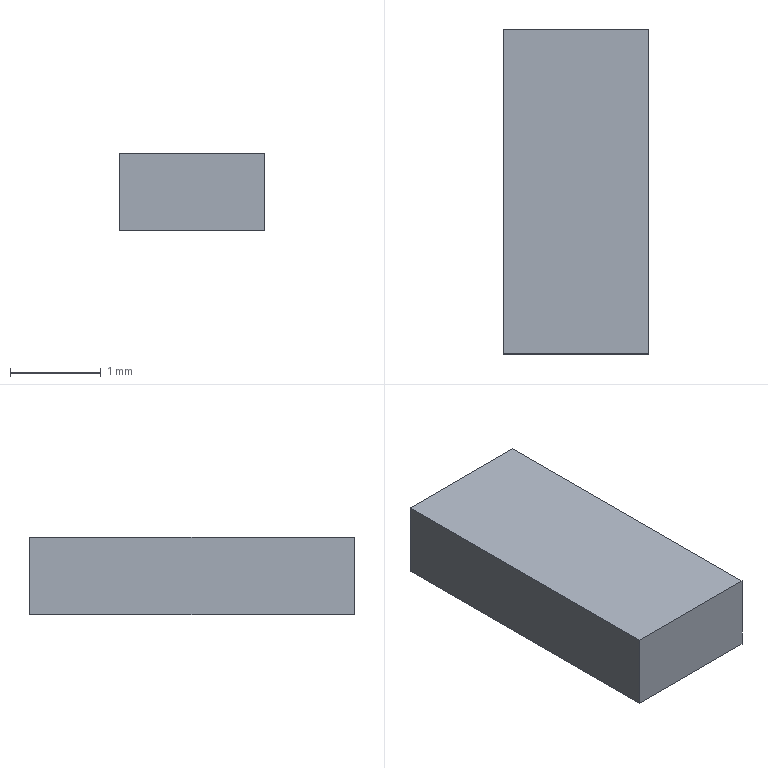Part | Creo | 1 solid | 6 faces | box 1.6 x 3.567 x 0.8499 mm | volume 4.85 mm3 | plane 6
STEP:
#1=CARTESIAN_POINT('',(0.,0.,0.));
#2=DIRECTION('',(0.,0.,1.));
#3=DIRECTION('',(1.,0.,0.));
#4=AXIS2_PLACEMENT_3D('',#1,#2,#3);
#5=CARTESIAN_POINT('',(-0.8,-1.783,0.));
#6=VERTEX_POINT('',#5);
#7=CARTESIAN_POINT('',(0.8,-1.783,0.));
#8=VERTEX_POINT('',#7);
#9=CARTESIAN_POINT('',(-0.8,-1.783,0.));
#10=DIRECTION('',(1.,0.,0.));
#11=VECTOR('',#10,1.6);
#12=LINE('',#9,#11);
#13=EDGE_CURVE('',#6,#8,#12,.T.);
#14=ORIENTED_EDGE('',*,*,#13,.T.);
#15=CARTESIAN_POINT('',(0.8,1.783,0.));
#16=VERTEX_POINT('',#15);
#17=CARTESIAN_POINT('',(0.8,-1.783,0.));
#18=DIRECTION('',(0.,1.,0.));
#19=VECTOR('',#18,3.567);
#20=LINE('',#17,#19);
#21=EDGE_CURVE('',#8,#16,#20,.T.);
#22=ORIENTED_EDGE('',*,*,#21,.T.);
#23=CARTESIAN_POINT('',(-0.8,1.783,0.));
#24=VERTEX_POINT('',#23);
#25=CARTESIAN_POINT('',(0.8,1.783,0.));
#26=DIRECTION('',(-1.,0.,0.));
#27=VECTOR('',#26,1.6);
#28=LINE('',#25,#27);
#29=EDGE_CURVE('',#16,#24,#28,.T.);
#30=ORIENTED_EDGE('',*,*,#29,.T.);
#31=CARTESIAN_POINT('',(-0.8,1.783,0.));
#32=DIRECTION('',(0.,-1.,0.));
#33=VECTOR('',#32,3.567);
#34=LINE('',#31,#33);
#35=EDGE_CURVE('',#24,#6,#34,.T.);
#36=ORIENTED_EDGE('',*,*,#35,.T.);
#37=EDGE_LOOP('',(#14,#22,#30,#36));
#38=FACE_OUTER_BOUND('',#37,.F.);
#39=CARTESIAN_POINT('',(0.,0.,0.));
#40=DIRECTION('',(0.,0.,1.));
#41=DIRECTION('',(1.,0.,0.));
#42=AXIS2_PLACEMENT_3D('',#39,#40,#41);
#43=PLANE('',#42);
#44=ADVANCED_FACE('',(#38),#43,.F.);
#45=ORIENTED_EDGE('',*,*,#13,.F.);
#46=CARTESIAN_POINT('',(-0.8,-1.783,0.8499));
#47=VERTEX_POINT('',#46);
#48=CARTESIAN_POINT('',(-0.8,-1.783,0.));
#49=DIRECTION('',(0.,0.,1.));
#50=VECTOR('',#49,0.8499);
#51=LINE('',#48,#50);
#52=EDGE_CURVE('',#6,#47,#51,.T.);
#53=ORIENTED_EDGE('',*,*,#52,.T.);
#54=CARTESIAN_POINT('',(0.8,-1.783,0.8499));
#55=VERTEX_POINT('',#54);
#56=CARTESIAN_POINT('',(-0.8,-1.783,0.8499));
#57=DIRECTION('',(1.,0.,0.));
#58=VECTOR('',#57,1.6);
#59=LINE('',#56,#58);
#60=EDGE_CURVE('',#47,#55,#59,.T.);
#61=ORIENTED_EDGE('',*,*,#60,.T.);
#62=CARTESIAN_POINT('',(0.8,-1.783,0.));
#63=DIRECTION('',(0.,0.,1.));
#64=VECTOR('',#63,0.8499);
#65=LINE('',#62,#64);
#66=EDGE_CURVE('',#8,#55,#65,.T.);
#67=ORIENTED_EDGE('',*,*,#66,.F.);
#68=EDGE_LOOP('',(#45,#53,#61,#67));
#69=FACE_OUTER_BOUND('',#68,.F.);
#70=CARTESIAN_POINT('',(-0.8,-1.783,0.));
#71=DIRECTION('',(0.,-1.,0.));
#72=DIRECTION('',(1.,0.,0.));
#73=AXIS2_PLACEMENT_3D('',#70,#71,#72);
#74=PLANE('',#73);
#75=ADVANCED_FACE('',(#69),#74,.T.);
#76=ORIENTED_EDGE('',*,*,#35,.F.);
#77=CARTESIAN_POINT('',(-0.8,1.783,0.8499));
#78=VERTEX_POINT('',#77);
#79=CARTESIAN_POINT('',(-0.8,1.783,0.));
#80=DIRECTION('',(0.,0.,1.));
#81=VECTOR('',#80,0.8499);
#82=LINE('',#79,#81);
#83=EDGE_CURVE('',#24,#78,#82,.T.);
#84=ORIENTED_EDGE('',*,*,#83,.T.);
#85=CARTESIAN_POINT('',(-0.8,1.783,0.8499));
#86=DIRECTION('',(0.,-1.,0.));
#87=VECTOR('',#86,3.567);
#88=LINE('',#85,#87);
#89=EDGE_CURVE('',#78,#47,#88,.T.);
#90=ORIENTED_EDGE('',*,*,#89,.T.);
#91=ORIENTED_EDGE('',*,*,#52,.F.);
#92=EDGE_LOOP('',(#76,#84,#90,#91));
#93=FACE_OUTER_BOUND('',#92,.F.);
#94=CARTESIAN_POINT('',(-0.8,1.783,0.));
#95=DIRECTION('',(-1.,0.,0.));
#96=DIRECTION('',(0.,-1.,0.));
#97=AXIS2_PLACEMENT_3D('',#94,#95,#96);
#98=PLANE('',#97);
#99=ADVANCED_FACE('',(#93),#98,.T.);
#100=ORIENTED_EDGE('',*,*,#29,.F.);
#101=CARTESIAN_POINT('',(0.8,1.783,0.8499));
#102=VERTEX_POINT('',#101);
#103=CARTESIAN_POINT('',(0.8,1.783,0.));
#104=DIRECTION('',(0.,0.,1.));
#105=VECTOR('',#104,0.8499);
#106=LINE('',#103,#105);
#107=EDGE_CURVE('',#16,#102,#106,.T.);
#108=ORIENTED_EDGE('',*,*,#107,.T.);
#109=CARTESIAN_POINT('',(0.8,1.783,0.8499));
#110=DIRECTION('',(-1.,0.,0.));
#111=VECTOR('',#110,1.6);
#112=LINE('',#109,#111);
#113=EDGE_CURVE('',#102,#78,#112,.T.);
#114=ORIENTED_EDGE('',*,*,#113,.T.);
#115=ORIENTED_EDGE('',*,*,#83,.F.);
#116=EDGE_LOOP('',(#100,#108,#114,#115));
#117=FACE_OUTER_BOUND('',#116,.F.);
#118=CARTESIAN_POINT('',(0.8,1.783,0.));
#119=DIRECTION('',(0.,1.,0.));
#120=DIRECTION('',(-1.,0.,0.));
#121=AXIS2_PLACEMENT_3D('',#118,#119,#120);
#122=PLANE('',#121);
#123=ADVANCED_FACE('',(#117),#122,.T.);
#124=ORIENTED_EDGE('',*,*,#21,.F.);
#125=ORIENTED_EDGE('',*,*,#66,.T.);
#126=CARTESIAN_POINT('',(0.8,-1.783,0.8499));
#127=DIRECTION('',(0.,1.,0.));
#128=VECTOR('',#127,3.567);
#129=LINE('',#126,#128);
#130=EDGE_CURVE('',#55,#102,#129,.T.);
#131=ORIENTED_EDGE('',*,*,#130,.T.);
#132=ORIENTED_EDGE('',*,*,#107,.F.);
#133=EDGE_LOOP('',(#124,#125,#131,#132));
#134=FACE_OUTER_BOUND('',#133,.F.);
#135=CARTESIAN_POINT('',(0.8,-1.783,0.));
#136=DIRECTION('',(1.,0.,0.));
#137=DIRECTION('',(0.,1.,0.));
#138=AXIS2_PLACEMENT_3D('',#135,#136,#137);
#139=PLANE('',#138);
#140=ADVANCED_FACE('',(#134),#139,.T.);
#141=ORIENTED_EDGE('',*,*,#60,.F.);
#142=ORIENTED_EDGE('',*,*,#89,.F.);
#143=ORIENTED_EDGE('',*,*,#113,.F.);
#144=ORIENTED_EDGE('',*,*,#130,.F.);
#145=EDGE_LOOP('',(#141,#142,#143,#144));
#146=FACE_OUTER_BOUND('',#145,.F.);
#147=CARTESIAN_POINT('',(0.,0.,0.8499));
#148=DIRECTION('',(0.,0.,1.));
#149=DIRECTION('',(1.,0.,0.));
#150=AXIS2_PLACEMENT_3D('',#147,#148,#149);
#151=PLANE('',#150);
#152=ADVANCED_FACE('',(#146),#151,.T.);
#153=CLOSED_SHELL('',(#44,#75,#99,#123,#140,#152));
#154=MANIFOLD_SOLID_BREP('',#153);
#155=(LENGTH_UNIT()NAMED_UNIT(*)SI_UNIT(.MILLI.,.METRE.));
#156=UNCERTAINTY_MEASURE_WITH_UNIT(LENGTH_MEASURE(0.0004),#155,'','');
#157=(NAMED_UNIT(*)PLANE_ANGLE_UNIT()SI_UNIT($,.RADIAN.));
#158=PLANE_ANGLE_MEASURE_WITH_UNIT(PLANE_ANGLE_MEASURE(0.01745),#157);
#159=(CONVERSION_BASED_UNIT('DEGREE',#158)NAMED_UNIT(*)PLANE_ANGLE_UNIT());
#160=(NAMED_UNIT(*)SI_UNIT($,.STERADIAN.)SOLID_ANGLE_UNIT());
#161=(GEOMETRIC_REPRESENTATION_CONTEXT(3)GLOBAL_UNCERTAINTY_ASSIGNED_CONTEXT((#156))GLOBAL_UNIT_ASSIGNED_CONTEXT((#155,#159,#160))REPRESENTATION_CONTEXT('',''));
#162=ADVANCED_BREP_SHAPE_REPRESENTATION('',(#4,#154),#161);